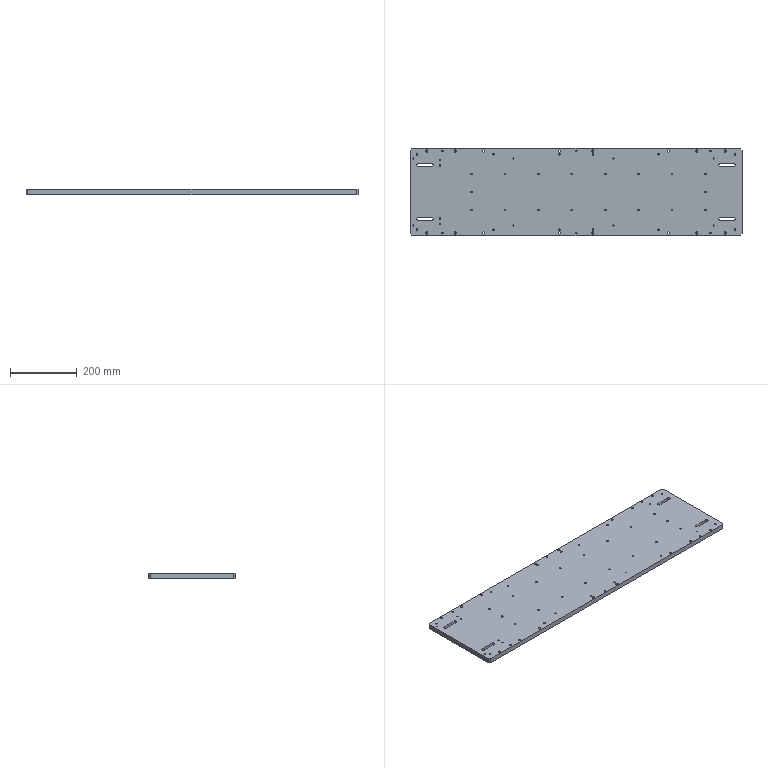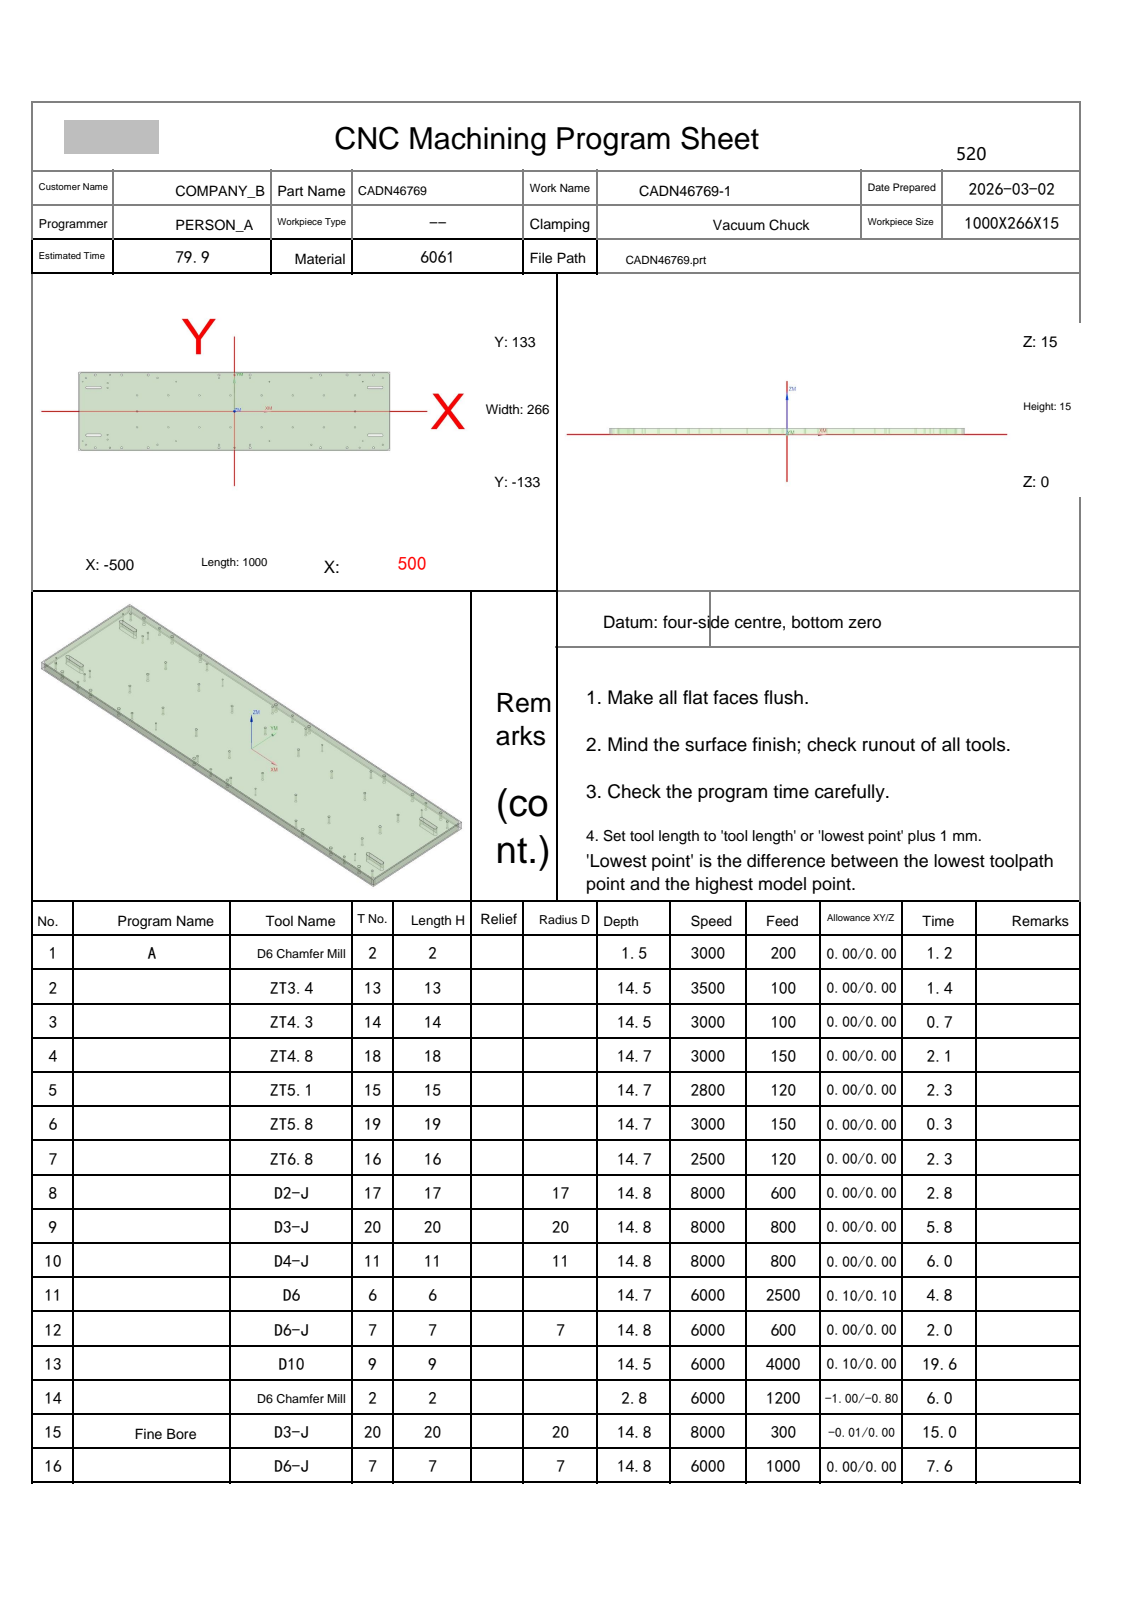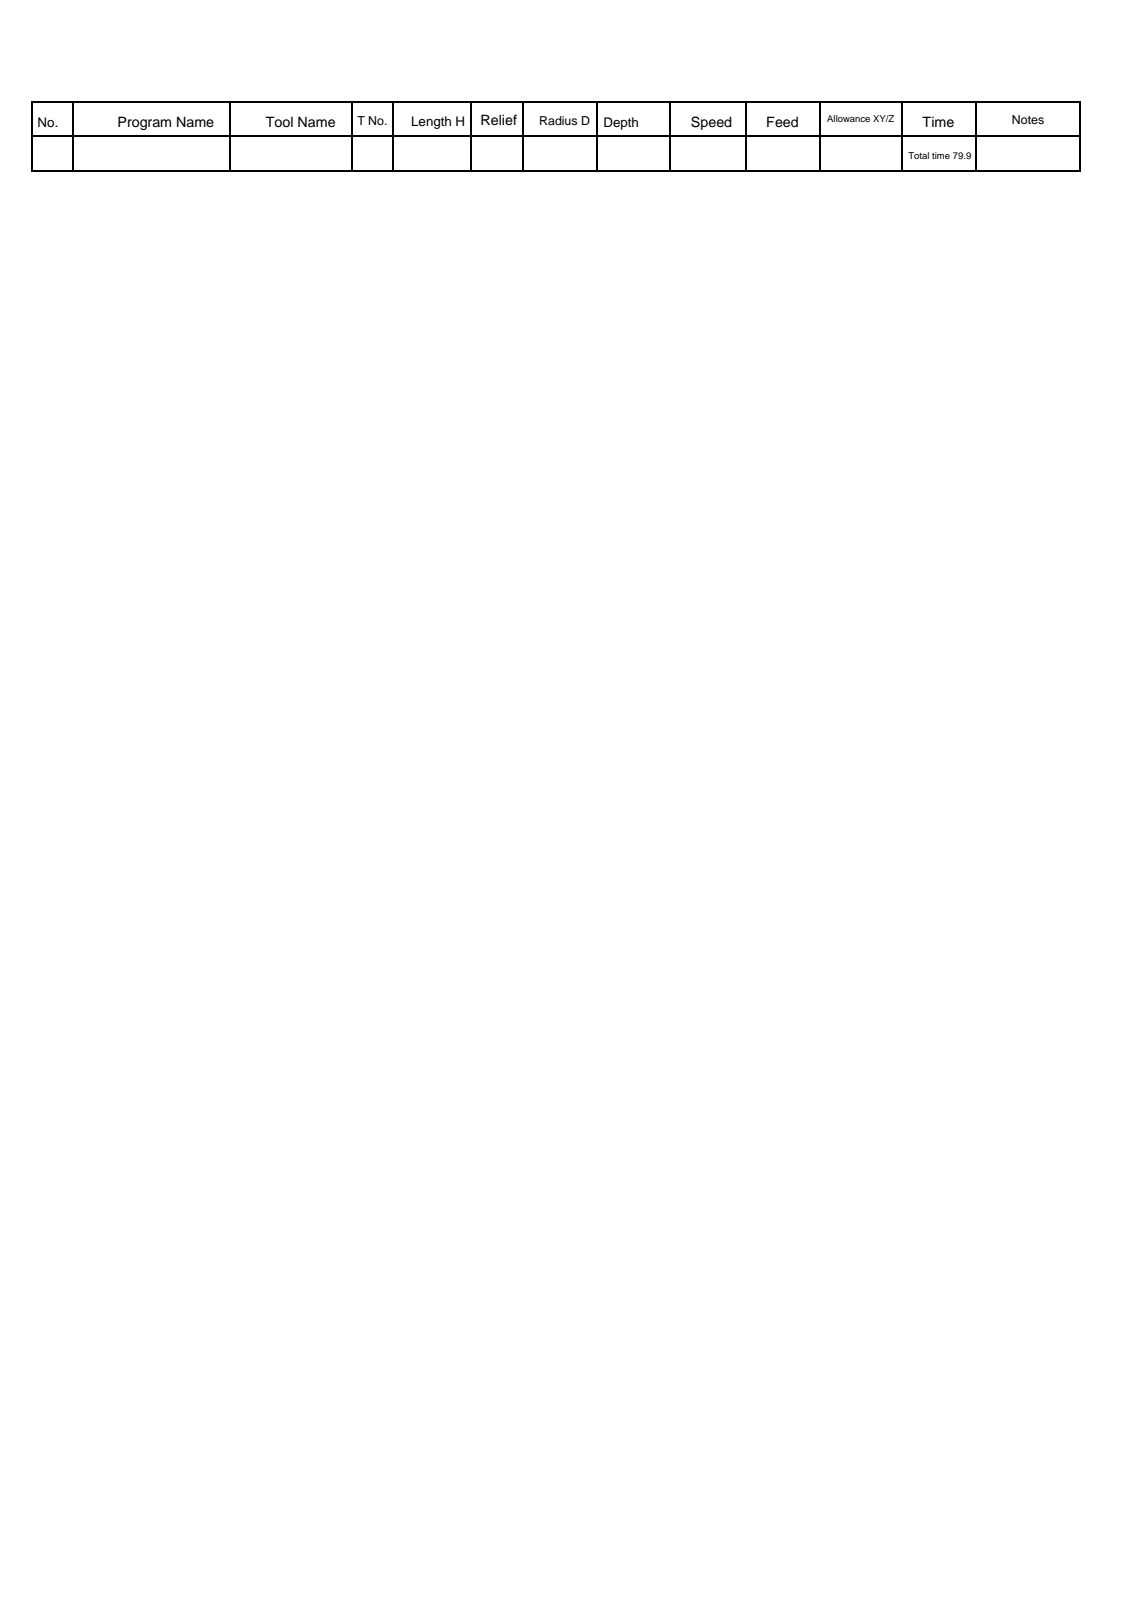NC program | NX | posted by the shop | part box 995 x 261 x 15 mm
Lines 1 to 234 of 14350:
%
O0001
(Machine time: 82.53 MIN)
(===Total Tool:13===)
(T2=D6 Chamfer Mill   D=6.   R=0.   D-  H02 Z=12.2  )
(T13=ZT3.4  D=3.4  DR_a=118 D-  H13 Z=0.5   )
(T14=ZT4.3  D=4.3  DR_a=118 D-  H14 Z=0.5   )
(T18=ZT4.8  D=4.8  DR_a=118 D-  H18 Z=0.3   )
(T15=ZT5.1  D=5.1  DR_a=118 D-  H15 Z=0.3   )
(T19=ZT5.8  D=5.8  DR_a=118 D-  H19 Z=0.3   )
(T16=ZT6.8  D=6.8  DR_a=118 D-  H16 Z=0.3   )
(T17=D2-J   D=2.   R=0.   D17 H17 Z=0.2   )
(T20=D3-J   D=3.   R=0.   D20 H20 Z=0.2   )
(T11=D4-J   D=4.   R=0.   D11 H11 Z=0.2   )
(T6=D6      D=6.   R=0.   D-  H06 Z=0.3   )
(T7=D6-J    D=6.   R=0.   D7  H07 Z=0.2   )
(T9=D10     D=10.  R=0.   D-  H09 Z=0.5   )
G80 G90 G17 G49 G40
G91 G28 Z0
M01
N1 T02 M06
(D6 Chamfer Mill  D=6. R=0. H=02 ce=0.00 di=0.00)
G00 G90 G54 X477. Y113. M03 S3000
G43 H02 Z45.
M08
G98 G81 X477. Y113. Z13.5 R16. F200.
X447. Y123.
X412.5 Y100.5
X402.5 Y123.
X362.
X387.5 Y54.
Y0.0
Y-54.
X412.5 Y-100.5
X477. Y-113.
X447. Y-123.
X402.5
X362.
X277.
X247. Y-113.
X287.5 Y-54.
X187.5
X112.5 Y-100.5
X87.5 Y-54.
X50.5 Y-113.
Y-123.
X.5
X-49.5
Y-113.
X-12.5 Y-54.
X-112.5
X-187.5 Y-100.5
X-212.5 Y-54.
X-247. Y-113.
X-277. Y-123.
X-362.
X-400.
X-447.
X-477. Y-113.
X-487.5 Y-100.5
X-407.5 Y-95.5
Y-79.5
X-312.5 Y-54.
Y0.0
Y54.
X-407.5 Y79.5
Y95.5
X-487.5 Y100.5
X-477. Y113.
X-447. Y123.
X-400.
X-362.
X-277.
X-247. Y113.
X-212.5 Y54.
X-187.5 Y100.5
X-112.5 Y54.
X-12.5
X-49.5 Y113.
Y123.
X.5
X50.5
Y113.
X87.5 Y54.
X112.5 Y100.5
X187.5 Y54.
X247. Y113.
X277. Y123.
X287.5 Y54.
G80
G00 Z45.
G91 G28 Z0.0
M05
M09
G91 G28 Z0.0
M01
N2 T13 M06
(ZT3.4 D=3.4 DR_a=118 H=13)
G00 G90 G54 X-487.5 Y-100.5 M03 S3500
G43 H13 Z45.
M08
G98 G83 X-487.5 Y-100.5 Z.5 R16. F100. Q1.5
Y100.5
X-187.5
Y-100.5
X112.5
Y100.5
X412.5
Y-100.5
G80
G00 Z45.
G91 G28 Z0.0
M05
M09
G91 G28 Z0.0
M01
N3 T14 M06
(ZT4.3 D=4.3 DR_a=118 H=14)
G00 G90 G54 X-407.5 Y-95.5 M03 S3000
G43 H14 Z45.
M08
G98 G83 X-407.5 Y-95.5 Z.5 R16. F100. Q1.5
Y-79.5
Y79.5
Y95.5
G80
G00 Z45.
G91 G28 Z0.0
M05
M09
G91 G28 Z0.0
M01
N4 T18 M06
(ZT4.8 D=4.8 DR_a=118 H=18)
G00 G90 G54 X477. Y113. M03 S3000
G43 H18 Z45.
M08
G98 G83 X477. Y113. Z.3 R16. F150. Q3.
X402.5 Y123.
X247. Y113.
X50.5
X.5 Y123.
X-49.5 Y113.
X-247.
X-400. Y123.
X-477. Y113.
Y-113.
X-400. Y-123.
X-247. Y-113.
X-49.5
X.5 Y-123.
X50.5 Y-113.
X247.
X402.5 Y-123.
X477. Y-113.
G80
G00 Z45.
G91 G28 Z0.0
M05
M09
G91 G28 Z0.0
M01
N5 T15 M06
(ZT5.1 D=5.1 DR_a=118 H=15)
G00 G90 G54 X387.5 Y-54. M03 S2800
G43 H15 Z45.
M08
G98 G83 X387.5 Y-54. Z.3 R16. F120. Q1.5
X287.5
X187.5
X87.5
X-12.5
X-112.5
X-212.5
X-312.5
Y54.
X-212.5
X-112.5
X-12.5
X87.5
X187.5
X287.5
X387.5
G80
G00 Z45.
G91 G28 Z0.0
M05
M09
G91 G28 Z0.0
M01
N6 T19 M06
(ZT5.8 D=5.8 DR_a=118 H=19)
G00 G90 G54 X387.5 Y0.0 M03 S3000
G43 H19 Z45.
M08
G98 G83 X387.5 Y0.0 Z.3 R16. F150. Q3.
X-312.5
G80
G00 Z45.
G91 G28 Z0.0
M05
M09
G91 G28 Z0.0
M01
N7 T16 M06
(ZT6.8 D=6.8 DR_a=118 H=16)
G00 G90 G54 X-447. Y-123. M03 S2500
G43 H16 Z45.
M08
G98 G83 X-447. Y-123. Z.3 R16. F120. Q1.5
X-362.
X-277.
X-49.5
X50.5
X277.
X362.
X447.
Y123.
X362.
X277.
X50.5
X-49.5
X-277.
X-362.
X-447.
G80
G00 Z45.
G91 G28 Z0.0
M05
M09
G91 G28 Z0.0
M01